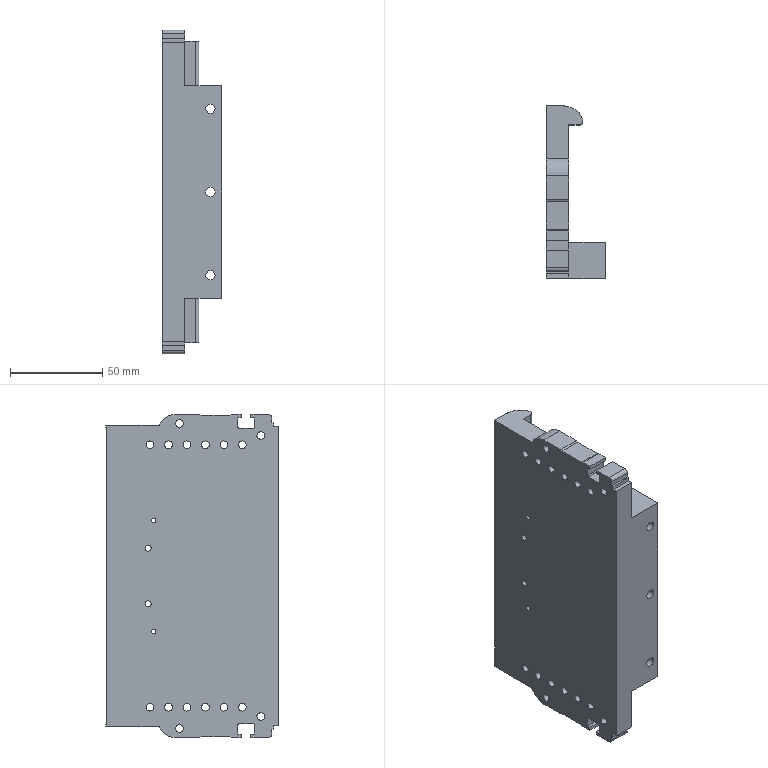Part | SolidWorks | features BaseBody 1 | 1 solid | 119 faces | box 32 x 93.5 x 175 mm | volume 238017 mm3 | cylinder 64 | plane 55 | commonest cylinder face diameters 4.2 x32 8 x8 5 x6 1 x4 2.5 x4 3.3 x4